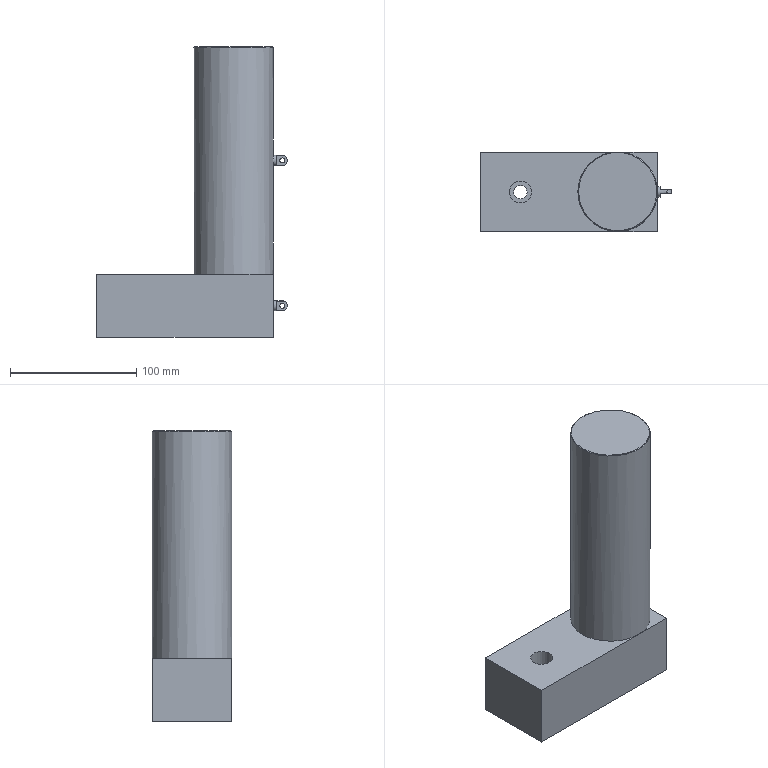Part | NX | features solid 2 | 1 solid | 37 faces | box 151 x 63 x 230 mm | volume 983981 mm3 | plane 23 | cylinder 13 | cone 1 | commonest cylinder face diameters 8 x4 4 x2 10.5 x2 17.5 x2 6 x1 10 x1
STEP:
#1=CARTESIAN_POINT('',(1540.,-559.,95.));
#2=VERTEX_POINT('',#1);
#3=CARTESIAN_POINT('',(1540.,-527.5,95.));
#4=VERTEX_POINT('',#3);
#5=CARTESIAN_POINT('',(1540.,-509.,95.));
#6=DIRECTION('',(0.,1.,0.));
#7=VECTOR('',#6,1000.);
#8=LINE('',#5,#7);
#9=EDGE_CURVE('',#2,#4,#8,.T.);
#10=ORIENTED_EDGE('',*,*,#9,.F.);
#11=CARTESIAN_POINT('',(1540.,-559.,45.));
#12=VERTEX_POINT('',#11);
#13=CARTESIAN_POINT('',(1540.,-559.,45.));
#14=DIRECTION('',(0.,0.,1.));
#15=VECTOR('',#14,1000.);
#16=LINE('',#13,#15);
#17=EDGE_CURVE('',#12,#2,#16,.T.);
#18=ORIENTED_EDGE('',*,*,#17,.F.);
#19=CARTESIAN_POINT('',(1540.,-496.,45.));
#20=VERTEX_POINT('',#19);
#21=CARTESIAN_POINT('',(1540.,-509.,45.));
#22=DIRECTION('',(0.,-1.,0.));
#23=VECTOR('',#22,1000.);
#24=LINE('',#21,#23);
#25=EDGE_CURVE('',#20,#12,#24,.T.);
#26=ORIENTED_EDGE('',*,*,#25,.F.);
#27=CARTESIAN_POINT('',(1540.,-496.,95.));
#28=VERTEX_POINT('',#27);
#29=CARTESIAN_POINT('',(1540.,-496.,203.412));
#30=DIRECTION('',(0.,0.,1.));
#31=VECTOR('',#30,1000.);
#32=LINE('',#29,#31);
#33=EDGE_CURVE('',#20,#28,#32,.T.);
#34=ORIENTED_EDGE('',*,*,#33,.T.);
#35=CARTESIAN_POINT('',(1540.,-509.,95.));
#36=DIRECTION('',(0.,1.,0.));
#37=VECTOR('',#36,1000.);
#38=LINE('',#35,#37);
#39=EDGE_CURVE('',#4,#28,#38,.T.);
#40=ORIENTED_EDGE('',*,*,#39,.F.);
#41=EDGE_LOOP('',(#10,#18,#26,#34,#40));
#42=FACE_BOUND('',#41,.T.);
#43=CARTESIAN_POINT('',(1540.,-523.5,70.));
#44=VERTEX_POINT('',#43);
#45=CARTESIAN_POINT('',(1540.,-527.5,70.));
#46=DIRECTION('',(1.,0.,0.));
#47=DIRECTION('',(0.,1.,0.));
#48=AXIS2_PLACEMENT_3D('',#45,#46,#47);
#49=CIRCLE('',#48,4.);
#50=EDGE_CURVE('',#44,#44,#49,.F.);
#51=ORIENTED_EDGE('',*,*,#50,.T.);
#52=EDGE_LOOP('',(#51));
#53=FACE_BOUND('',#52,.T.);
#54=CARTESIAN_POINT('',(1540.,-509.,45.));
#55=DIRECTION('',(1.,0.,0.));
#56=DIRECTION('',(0.,1.,0.));
#57=AXIS2_PLACEMENT_3D('',#54,#55,#56);
#58=PLANE('',#57);
#59=ADVANCED_FACE('',(#42,#53),#58,.T.);
#60=ORIENTED_EDGE('',*,*,#9,.T.);
#61=CARTESIAN_POINT('',(1508.5,-559.,95.));
#62=VERTEX_POINT('',#61);
#63=CARTESIAN_POINT('',(1508.5,-527.5,95.));
#64=DIRECTION('',(0.,0.,-1.));
#65=DIRECTION('',(1.,0.,0.));
#66=AXIS2_PLACEMENT_3D('',#63,#64,#65);
#67=CIRCLE('',#66,31.5);
#68=EDGE_CURVE('',#4,#62,#67,.T.);
#69=ORIENTED_EDGE('',*,*,#68,.T.);
#70=CARTESIAN_POINT('',(1263.352,-559.,95.));
#71=DIRECTION('',(1.,0.,0.));
#72=VECTOR('',#71,1000.);
#73=LINE('',#70,#72);
#74=EDGE_CURVE('',#62,#2,#73,.T.);
#75=ORIENTED_EDGE('',*,*,#74,.T.);
#76=EDGE_LOOP('',(#60,#69,#75));
#77=FACE_BOUND('',#76,.T.);
#78=CARTESIAN_POINT('',(1470.,-527.5,95.));
#79=DIRECTION('',(0.,0.,-1.));
#80=DIRECTION('',(1.,0.,0.));
#81=AXIS2_PLACEMENT_3D('',#78,#79,#80);
#82=PLANE('',#81);
#83=ADVANCED_FACE('',(#77),#82,.F.);
#84=CARTESIAN_POINT('',(1422.75,-527.5,95.));
#85=VERTEX_POINT('',#84);
#86=CARTESIAN_POINT('',(1431.5,-527.5,95.));
#87=DIRECTION('',(0.,0.,1.));
#88=DIRECTION('',(-1.,0.,0.));
#89=AXIS2_PLACEMENT_3D('',#86,#87,#88);
#90=CIRCLE('',#89,8.75);
#91=EDGE_CURVE('',#85,#85,#90,.F.);
#92=ORIENTED_EDGE('',*,*,#91,.T.);
#93=EDGE_LOOP('',(#92));
#94=FACE_BOUND('',#93,.T.);
#95=CARTESIAN_POINT('',(1400.,-559.,95.));
#96=VERTEX_POINT('',#95);
#97=CARTESIAN_POINT('',(1263.352,-559.,95.));
#98=DIRECTION('',(1.,0.,0.));
#99=VECTOR('',#98,1000.);
#100=LINE('',#97,#99);
#101=EDGE_CURVE('',#96,#62,#100,.T.);
#102=ORIENTED_EDGE('',*,*,#101,.T.);
#103=CARTESIAN_POINT('',(1508.5,-496.,95.));
#104=VERTEX_POINT('',#103);
#105=CARTESIAN_POINT('',(1508.5,-527.5,95.));
#106=DIRECTION('',(0.,0.,-1.));
#107=DIRECTION('',(1.,0.,0.));
#108=AXIS2_PLACEMENT_3D('',#105,#106,#107);
#109=CIRCLE('',#108,31.5);
#110=EDGE_CURVE('',#62,#104,#109,.T.);
#111=ORIENTED_EDGE('',*,*,#110,.T.);
#112=CARTESIAN_POINT('',(1400.,-496.,95.));
#113=VERTEX_POINT('',#112);
#114=CARTESIAN_POINT('',(1263.352,-496.,95.));
#115=DIRECTION('',(1.,0.,0.));
#116=VECTOR('',#115,1000.);
#117=LINE('',#114,#116);
#118=EDGE_CURVE('',#113,#104,#117,.T.);
#119=ORIENTED_EDGE('',*,*,#118,.F.);
#120=CARTESIAN_POINT('',(1400.,-509.,95.));
#121=DIRECTION('',(0.,1.,0.));
#122=VECTOR('',#121,1000.);
#123=LINE('',#120,#122);
#124=EDGE_CURVE('',#96,#113,#123,.T.);
#125=ORIENTED_EDGE('',*,*,#124,.F.);
#126=EDGE_LOOP('',(#102,#111,#119,#125));
#127=FACE_BOUND('',#126,.T.);
#128=CARTESIAN_POINT('',(1470.,-527.5,95.));
#129=DIRECTION('',(0.,0.,-1.));
#130=DIRECTION('',(1.,0.,0.));
#131=AXIS2_PLACEMENT_3D('',#128,#129,#130);
#132=PLANE('',#131);
#133=ADVANCED_FACE('',(#94,#127),#132,.F.);
#134=CARTESIAN_POINT('',(1400.,-496.,45.));
#135=VERTEX_POINT('',#134);
#136=CARTESIAN_POINT('',(1263.352,-496.,45.));
#137=DIRECTION('',(1.,0.,0.));
#138=VECTOR('',#137,1000.);
#139=LINE('',#136,#138);
#140=EDGE_CURVE('',#135,#20,#139,.T.);
#141=ORIENTED_EDGE('',*,*,#140,.F.);
#142=CARTESIAN_POINT('',(1400.,-496.,203.412));
#143=DIRECTION('',(0.,0.,1.));
#144=VECTOR('',#143,1000.);
#145=LINE('',#142,#144);
#146=EDGE_CURVE('',#135,#113,#145,.T.);
#147=ORIENTED_EDGE('',*,*,#146,.T.);
#148=ORIENTED_EDGE('',*,*,#118,.T.);
#149=CARTESIAN_POINT('',(1263.352,-496.,95.));
#150=DIRECTION('',(1.,0.,0.));
#151=VECTOR('',#150,1000.);
#152=LINE('',#149,#151);
#153=EDGE_CURVE('',#104,#28,#152,.T.);
#154=ORIENTED_EDGE('',*,*,#153,.T.);
#155=ORIENTED_EDGE('',*,*,#33,.F.);
#156=EDGE_LOOP('',(#141,#147,#148,#154,#155));
#157=FACE_BOUND('',#156,.T.);
#158=CARTESIAN_POINT('',(1263.352,-496.,203.412));
#159=DIRECTION('',(0.,-1.,0.));
#160=DIRECTION('',(1.,0.,0.));
#161=AXIS2_PLACEMENT_3D('',#158,#159,#160);
#162=PLANE('',#161);
#163=ADVANCED_FACE('',(#157),#162,.F.);
#164=ORIENTED_EDGE('',*,*,#101,.F.);
#165=CARTESIAN_POINT('',(1400.,-559.,45.));
#166=VERTEX_POINT('',#165);
#167=CARTESIAN_POINT('',(1400.,-559.,45.));
#168=DIRECTION('',(0.,0.,1.));
#169=VECTOR('',#168,1000.);
#170=LINE('',#167,#169);
#171=EDGE_CURVE('',#166,#96,#170,.T.);
#172=ORIENTED_EDGE('',*,*,#171,.F.);
#173=CARTESIAN_POINT('',(1263.352,-559.,45.));
#174=DIRECTION('',(1.,0.,0.));
#175=VECTOR('',#174,1000.);
#176=LINE('',#173,#175);
#177=EDGE_CURVE('',#166,#12,#176,.T.);
#178=ORIENTED_EDGE('',*,*,#177,.T.);
#179=ORIENTED_EDGE('',*,*,#17,.T.);
#180=ORIENTED_EDGE('',*,*,#74,.F.);
#181=EDGE_LOOP('',(#164,#172,#178,#179,#180));
#182=FACE_BOUND('',#181,.T.);
#183=CARTESIAN_POINT('',(1263.352,-559.,203.412));
#184=DIRECTION('',(0.,-1.,0.));
#185=DIRECTION('',(1.,0.,0.));
#186=AXIS2_PLACEMENT_3D('',#183,#184,#185);
#187=PLANE('',#186);
#188=ADVANCED_FACE('',(#182),#187,.T.);
#189=CARTESIAN_POINT('',(1513.75,-527.5,45.));
#190=VERTEX_POINT('',#189);
#191=CARTESIAN_POINT('',(1508.5,-527.5,45.));
#192=DIRECTION('',(0.,0.,-1.));
#193=DIRECTION('',(1.,0.,0.));
#194=AXIS2_PLACEMENT_3D('',#191,#192,#193);
#195=CIRCLE('',#194,5.25);
#196=EDGE_CURVE('',#190,#190,#195,.F.);
#197=ORIENTED_EDGE('',*,*,#196,.T.);
#198=EDGE_LOOP('',(#197));
#199=FACE_BOUND('',#198,.T.);
#200=ORIENTED_EDGE('',*,*,#25,.T.);
#201=ORIENTED_EDGE('',*,*,#177,.F.);
#202=CARTESIAN_POINT('',(1400.,-509.,45.));
#203=DIRECTION('',(0.,-1.,0.));
#204=VECTOR('',#203,1000.);
#205=LINE('',#202,#204);
#206=EDGE_CURVE('',#135,#166,#205,.T.);
#207=ORIENTED_EDGE('',*,*,#206,.F.);
#208=ORIENTED_EDGE('',*,*,#140,.T.);
#209=EDGE_LOOP('',(#200,#201,#207,#208));
#210=FACE_BOUND('',#209,.T.);
#211=CARTESIAN_POINT('',(1426.25,-527.5,45.));
#212=VERTEX_POINT('',#211);
#213=CARTESIAN_POINT('',(1431.5,-527.5,45.));
#214=DIRECTION('',(0.,0.,1.));
#215=DIRECTION('',(-1.,0.,0.));
#216=AXIS2_PLACEMENT_3D('',#213,#214,#215);
#217=CIRCLE('',#216,5.25);
#218=EDGE_CURVE('',#212,#212,#217,.F.);
#219=ORIENTED_EDGE('',*,*,#218,.F.);
#220=EDGE_LOOP('',(#219));
#221=FACE_BOUND('',#220,.T.);
#222=CARTESIAN_POINT('',(1263.352,-509.,45.));
#223=DIRECTION('',(0.,0.,-1.));
#224=DIRECTION('',(-1.,0.,0.));
#225=AXIS2_PLACEMENT_3D('',#222,#223,#224);
#226=PLANE('',#225);
#227=ADVANCED_FACE('',(#199,#210,#221),#226,.T.);
#228=ORIENTED_EDGE('',*,*,#153,.F.);
#229=CARTESIAN_POINT('',(1508.5,-527.5,95.));
#230=DIRECTION('',(0.,0.,-1.));
#231=DIRECTION('',(1.,0.,0.));
#232=AXIS2_PLACEMENT_3D('',#229,#230,#231);
#233=CIRCLE('',#232,31.5);
#234=EDGE_CURVE('',#104,#4,#233,.T.);
#235=ORIENTED_EDGE('',*,*,#234,.T.);
#236=ORIENTED_EDGE('',*,*,#39,.T.);
#237=EDGE_LOOP('',(#228,#235,#236));
#238=FACE_BOUND('',#237,.T.);
#239=CARTESIAN_POINT('',(1470.,-527.5,95.));
#240=DIRECTION('',(0.,0.,-1.));
#241=DIRECTION('',(1.,0.,0.));
#242=AXIS2_PLACEMENT_3D('',#239,#240,#241);
#243=PLANE('',#242);
#244=ADVANCED_FACE('',(#238),#243,.F.);
#245=CARTESIAN_POINT('',(1517.25,-527.5,65.));
#246=VERTEX_POINT('',#245);
#247=CARTESIAN_POINT('',(1508.5,-527.5,65.));
#248=DIRECTION('',(0.,0.,1.));
#249=DIRECTION('',(1.,0.,0.));
#250=AXIS2_PLACEMENT_3D('',#247,#248,#249);
#251=CIRCLE('',#250,8.75);
#252=EDGE_CURVE('',#246,#246,#251,.T.);
#253=ORIENTED_EDGE('',*,*,#252,.F.);
#254=EDGE_LOOP('',(#253));
#255=FACE_BOUND('',#254,.T.);
#256=CARTESIAN_POINT('',(1517.25,-527.5,95.));
#257=VERTEX_POINT('',#256);
#258=CARTESIAN_POINT('',(1508.5,-527.5,95.));
#259=DIRECTION('',(0.,0.,-1.));
#260=DIRECTION('',(1.,0.,0.));
#261=AXIS2_PLACEMENT_3D('',#258,#259,#260);
#262=CIRCLE('',#261,8.75);
#263=EDGE_CURVE('',#257,#257,#262,.F.);
#264=ORIENTED_EDGE('',*,*,#263,.T.);
#265=EDGE_LOOP('',(#264));
#266=FACE_BOUND('',#265,.T.);
#267=CARTESIAN_POINT('',(1508.5,-527.5,45.));
#268=DIRECTION('',(0.,0.,1.));
#269=DIRECTION('',(1.,0.,0.));
#270=AXIS2_PLACEMENT_3D('',#267,#268,#269);
#271=CYLINDRICAL_SURFACE('',#270,8.75);
#272=ADVANCED_FACE('',(#255,#266),#271,.F.);
#273=CARTESIAN_POINT('',(1513.75,-527.5,65.));
#274=VERTEX_POINT('',#273);
#275=CARTESIAN_POINT('',(1508.5,-527.5,65.));
#276=DIRECTION('',(0.,0.,-1.));
#277=DIRECTION('',(1.,0.,0.));
#278=AXIS2_PLACEMENT_3D('',#275,#276,#277);
#279=CIRCLE('',#278,5.25);
#280=EDGE_CURVE('',#274,#274,#279,.F.);
#281=ORIENTED_EDGE('',*,*,#280,.F.);
#282=EDGE_LOOP('',(#281));
#283=FACE_BOUND('',#282,.T.);
#284=ORIENTED_EDGE('',*,*,#252,.T.);
#285=EDGE_LOOP('',(#284));
#286=FACE_BOUND('',#285,.T.);
#287=CARTESIAN_POINT('',(1508.5,-527.5,65.));
#288=DIRECTION('',(0.,0.,-1.));
#289=DIRECTION('',(1.,0.,0.));
#290=AXIS2_PLACEMENT_3D('',#287,#288,#289);
#291=PLANE('',#290);
#292=ADVANCED_FACE('',(#283,#286),#291,.F.);
#293=ORIENTED_EDGE('',*,*,#196,.F.);
#294=EDGE_LOOP('',(#293));
#295=FACE_BOUND('',#294,.T.);
#296=ORIENTED_EDGE('',*,*,#280,.T.);
#297=EDGE_LOOP('',(#296));
#298=FACE_BOUND('',#297,.T.);
#299=CARTESIAN_POINT('',(1508.5,-527.5,65.));
#300=DIRECTION('',(0.,0.,-1.));
#301=DIRECTION('',(1.,0.,0.));
#302=AXIS2_PLACEMENT_3D('',#299,#300,#301);
#303=CYLINDRICAL_SURFACE('',#302,5.25);
#304=ADVANCED_FACE('',(#295,#298),#303,.F.);
#305=ORIENTED_EDGE('',*,*,#124,.T.);
#306=ORIENTED_EDGE('',*,*,#146,.F.);
#307=ORIENTED_EDGE('',*,*,#206,.T.);
#308=ORIENTED_EDGE('',*,*,#171,.T.);
#309=EDGE_LOOP('',(#305,#306,#307,#308));
#310=FACE_BOUND('',#309,.T.);
#311=CARTESIAN_POINT('',(1400.,-509.,45.));
#312=DIRECTION('',(-1.,0.,0.));
#313=DIRECTION('',(0.,1.,0.));
#314=AXIS2_PLACEMENT_3D('',#311,#312,#313);
#315=PLANE('',#314);
#316=ADVANCED_FACE('',(#310),#315,.T.);
#317=CARTESIAN_POINT('',(1422.75,-527.5,65.));
#318=VERTEX_POINT('',#317);
#319=CARTESIAN_POINT('',(1431.5,-527.5,65.));
#320=DIRECTION('',(0.,0.,-1.));
#321=DIRECTION('',(-1.,0.,0.));
#322=AXIS2_PLACEMENT_3D('',#319,#320,#321);
#323=CIRCLE('',#322,8.75);
#324=EDGE_CURVE('',#318,#318,#323,.T.);
#325=ORIENTED_EDGE('',*,*,#324,.T.);
#326=EDGE_LOOP('',(#325));
#327=FACE_BOUND('',#326,.T.);
#328=ORIENTED_EDGE('',*,*,#91,.F.);
#329=EDGE_LOOP('',(#328));
#330=FACE_BOUND('',#329,.T.);
#331=CARTESIAN_POINT('',(1431.5,-527.5,45.));
#332=DIRECTION('',(0.,0.,1.));
#333=DIRECTION('',(-1.,0.,0.));
#334=AXIS2_PLACEMENT_3D('',#331,#332,#333);
#335=CYLINDRICAL_SURFACE('',#334,8.75);
#336=ADVANCED_FACE('',(#327,#330),#335,.F.);
#337=CARTESIAN_POINT('',(1426.25,-527.5,65.));
#338=VERTEX_POINT('',#337);
#339=CARTESIAN_POINT('',(1431.5,-527.5,65.));
#340=DIRECTION('',(0.,0.,1.));
#341=DIRECTION('',(-1.,0.,0.));
#342=AXIS2_PLACEMENT_3D('',#339,#340,#341);
#343=CIRCLE('',#342,5.25);
#344=EDGE_CURVE('',#338,#338,#343,.F.);
#345=ORIENTED_EDGE('',*,*,#344,.T.);
#346=EDGE_LOOP('',(#345));
#347=FACE_BOUND('',#346,.T.);
#348=ORIENTED_EDGE('',*,*,#324,.F.);
#349=EDGE_LOOP('',(#348));
#350=FACE_BOUND('',#349,.T.);
#351=CARTESIAN_POINT('',(1431.5,-527.5,65.));
#352=DIRECTION('',(0.,0.,-1.));
#353=DIRECTION('',(-1.,0.,0.));
#354=AXIS2_PLACEMENT_3D('',#351,#352,#353);
#355=PLANE('',#354);
#356=ADVANCED_FACE('',(#347,#350),#355,.F.);
#357=ORIENTED_EDGE('',*,*,#218,.T.);
#358=EDGE_LOOP('',(#357));
#359=FACE_BOUND('',#358,.T.);
#360=ORIENTED_EDGE('',*,*,#344,.F.);
#361=EDGE_LOOP('',(#360));
#362=FACE_BOUND('',#361,.T.);
#363=CARTESIAN_POINT('',(1431.5,-527.5,65.));
#364=DIRECTION('',(0.,0.,-1.));
#365=DIRECTION('',(-1.,0.,0.));
#366=AXIS2_PLACEMENT_3D('',#363,#364,#365);
#367=CYLINDRICAL_SURFACE('',#366,5.25);
#368=ADVANCED_FACE('',(#359,#362),#367,.F.);
#369=CARTESIAN_POINT('',(1539.,-527.5,190.));
#370=VERTEX_POINT('',#369);
#371=CARTESIAN_POINT('',(1539.,-527.5,185.));
#372=DIRECTION('',(-1.,0.,0.));
#373=DIRECTION('',(0.,0.,1.));
#374=AXIS2_PLACEMENT_3D('',#371,#372,#373);
#375=CIRCLE('',#374,5.);
#376=EDGE_CURVE('',#370,#370,#375,.T.);
#377=ORIENTED_EDGE('',*,*,#376,.F.);
#378=EDGE_LOOP('',(#377));
#379=FACE_BOUND('',#378,.T.);
#380=CARTESIAN_POINT('',(1539.,-527.5,189.));
#381=VERTEX_POINT('',#380);
#382=CARTESIAN_POINT('',(1539.,-527.5,185.));
#383=DIRECTION('',(-1.,0.,0.));
#384=DIRECTION('',(0.,0.,1.));
#385=AXIS2_PLACEMENT_3D('',#382,#383,#384);
#386=CIRCLE('',#385,4.);
#387=EDGE_CURVE('',#381,#381,#386,.T.);
#388=ORIENTED_EDGE('',*,*,#387,.T.);
#389=EDGE_LOOP('',(#388));
#390=FACE_BOUND('',#389,.T.);
#391=CARTESIAN_POINT('',(1539.,-527.5,185.));
#392=DIRECTION('',(1.,0.,0.));
#393=DIRECTION('',(0.,0.,-1.));
#394=AXIS2_PLACEMENT_3D('',#391,#392,#393);
#395=PLANE('',#394);
#396=ADVANCED_FACE('',(#379,#390),#395,.T.);
#397=CARTESIAN_POINT('',(1540.,-527.5,274.5));
#398=VERTEX_POINT('',#397);
#399=CARTESIAN_POINT('',(1508.5,-527.5,274.5));
#400=DIRECTION('',(0.,0.,-1.));
#401=DIRECTION('',(1.,0.,0.));
#402=AXIS2_PLACEMENT_3D('',#399,#400,#401);
#403=CIRCLE('',#402,31.5);
#404=EDGE_CURVE('',#398,#398,#403,.F.);
#405=ORIENTED_EDGE('',*,*,#404,.F.);
#406=EDGE_LOOP('',(#405));
#407=FACE_BOUND('',#406,.T.);
#408=CARTESIAN_POINT('',(1540.,-527.5,180.));
#409=VERTEX_POINT('',#408);
#410=CARTESIAN_POINT('',(1539.801,-531.422,181.085));
#411=CARTESIAN_POINT('',(1540.099,-527.499,179.458));
#412=CARTESIAN_POINT('',(1539.801,-523.581,181.084));
#413=CARTESIAN_POINT('',(1539.5,-521.96,184.995));
#414=CARTESIAN_POINT('',(1539.801,-523.58,188.918));
#415=CARTESIAN_POINT('',(1540.099,-527.499,190.54));
#416=CARTESIAN_POINT('',(1539.802,-531.413,188.922));
#417=CARTESIAN_POINT('',(1539.5,-533.041,185.004));
#418=CARTESIAN_POINT('',(1539.801,-531.422,181.085));
#419=CARTESIAN_POINT('',(1540.099,-527.499,179.458));
#420=CARTESIAN_POINT('',(1539.801,-523.581,181.084));
#421=B_SPLINE_CURVE_WITH_KNOTS('',3,(#410,#411,#412,#413,#414,#415,#416,#417,#418,#419,#420),.UNSPECIFIED.,.T.,.F.,(1,1,1,1,1,1,1,1,1,1,1,1,1,1,1),(-0.01174,-0.007828,-0.003914,0.,0.003914,0.007828,0.01174,0.01566,0.01957,0.02348,0.0274,0.03131,0.03522,0.03914,0.04305),.UNSPECIFIED.);
#422=EDGE_CURVE('',#409,#409,#421,.T.);
#423=ORIENTED_EDGE('',*,*,#422,.F.);
#424=EDGE_LOOP('',(#423));
#425=FACE_BOUND('',#424,.T.);
#426=ORIENTED_EDGE('',*,*,#68,.F.);
#427=ORIENTED_EDGE('',*,*,#234,.F.);
#428=ORIENTED_EDGE('',*,*,#110,.F.);
#429=EDGE_LOOP('',(#426,#427,#428));
#430=FACE_BOUND('',#429,.T.);
#431=CARTESIAN_POINT('',(1508.5,-527.5,275.));
#432=DIRECTION('',(0.,0.,-1.));
#433=DIRECTION('',(-1.,0.,0.));
#434=AXIS2_PLACEMENT_3D('',#431,#432,#433);
#435=CYLINDRICAL_SURFACE('',#434,31.5);
#436=ADVANCED_FACE('',(#407,#425,#430),#435,.T.);
#437=CARTESIAN_POINT('',(1539.5,-527.5,275.));
#438=VERTEX_POINT('',#437);
#439=CARTESIAN_POINT('',(1508.5,-527.5,275.));
#440=DIRECTION('',(0.,0.,-1.));
#441=DIRECTION('',(1.,0.,0.));
#442=AXIS2_PLACEMENT_3D('',#439,#440,#441);
#443=CIRCLE('',#442,31.);
#444=EDGE_CURVE('',#438,#438,#443,.T.);
#445=ORIENTED_EDGE('',*,*,#444,.F.);
#446=EDGE_LOOP('',(#445));
#447=FACE_BOUND('',#446,.T.);
#448=CARTESIAN_POINT('',(1508.5,-527.5,275.));
#449=DIRECTION('',(0.,0.,1.));
#450=DIRECTION('',(1.,0.,0.));
#451=AXIS2_PLACEMENT_3D('',#448,#449,#450);
#452=PLANE('',#451);
#453=ADVANCED_FACE('',(#447),#452,.T.);
#454=ORIENTED_EDGE('',*,*,#376,.T.);
#455=EDGE_LOOP('',(#454));
#456=FACE_BOUND('',#455,.T.);
#457=ORIENTED_EDGE('',*,*,#422,.T.);
#458=EDGE_LOOP('',(#457));
#459=FACE_BOUND('',#458,.T.);
#460=CARTESIAN_POINT('',(1539.,-527.5,185.));
#461=DIRECTION('',(1.,0.,0.));
#462=DIRECTION('',(0.,0.,-1.));
#463=AXIS2_PLACEMENT_3D('',#460,#461,#462);
#464=CYLINDRICAL_SURFACE('',#463,5.);
#465=ADVANCED_FACE('',(#456,#459),#464,.F.);
#466=ORIENTED_EDGE('',*,*,#404,.T.);
#467=EDGE_LOOP('',(#466));
#468=FACE_BOUND('',#467,.T.);
#469=ORIENTED_EDGE('',*,*,#444,.T.);
#470=EDGE_LOOP('',(#469));
#471=FACE_BOUND('',#470,.T.);
#472=CARTESIAN_POINT('',(1508.5,-527.5,275.));
#473=DIRECTION('',(0.,0.,-1.));
#474=DIRECTION('',(-1.,0.,0.));
#475=AXIS2_PLACEMENT_3D('',#472,#473,#474);
#476=CONICAL_SURFACE('',#475,31.,0.7854);
#477=ADVANCED_FACE('',(#468,#471),#476,.T.);
#478=CARTESIAN_POINT('',(1548.5,-526.,181.292));
#479=VERTEX_POINT('',#478);
#480=CARTESIAN_POINT('',(1548.5,-526.,188.708));
#481=VERTEX_POINT('',#480);
#482=CARTESIAN_POINT('',(1547.,-526.,185.));
#483=DIRECTION('',(0.,-1.,0.));
#484=DIRECTION('',(1.,0.,0.));
#485=AXIS2_PLACEMENT_3D('',#482,#483,#484);
#486=CIRCLE('',#485,4.);
#487=EDGE_CURVE('',#479,#481,#486,.T.);
#488=ORIENTED_EDGE('',*,*,#487,.F.);
#489=CARTESIAN_POINT('',(1542.,-526.,181.292));
#490=VERTEX_POINT('',#489);
#491=CARTESIAN_POINT('',(1551.,-526.,181.292));
#492=DIRECTION('',(-1.,0.,0.));
#493=VECTOR('',#492,1000.);
#494=LINE('',#491,#493);
#495=EDGE_CURVE('',#490,#479,#494,.F.);
#496=ORIENTED_EDGE('',*,*,#495,.F.);
#497=CARTESIAN_POINT('',(1542.,-526.,188.708));
#498=VERTEX_POINT('',#497);
#499=CARTESIAN_POINT('',(1542.,-526.,189.));
#500=DIRECTION('',(0.,0.,-1.));
#501=VECTOR('',#500,1000.);
#502=LINE('',#499,#501);
#503=EDGE_CURVE('',#498,#490,#502,.T.);
#504=ORIENTED_EDGE('',*,*,#503,.F.);
#505=CARTESIAN_POINT('',(1551.,-526.,188.708));
#506=DIRECTION('',(-1.,0.,0.));
#507=VECTOR('',#506,1000.);
#508=LINE('',#505,#507);
#509=EDGE_CURVE('',#481,#498,#508,.T.);
#510=ORIENTED_EDGE('',*,*,#509,.F.);
#511=EDGE_LOOP('',(#488,#496,#504,#510));
#512=FACE_BOUND('',#511,.T.);
#513=CARTESIAN_POINT('',(1549.,-526.,185.));
#514=VERTEX_POINT('',#513);
#515=CARTESIAN_POINT('',(1547.,-526.,185.));
#516=DIRECTION('',(0.,-1.,0.));
#517=DIRECTION('',(1.,0.,0.));
#518=AXIS2_PLACEMENT_3D('',#515,#516,#517);
#519=CIRCLE('',#518,2.);
#520=EDGE_CURVE('',#514,#514,#519,.F.);
#521=ORIENTED_EDGE('',*,*,#520,.F.);
#522=EDGE_LOOP('',(#521));
#523=FACE_BOUND('',#522,.T.);
#524=CARTESIAN_POINT('',(1551.,-526.,189.));
#525=DIRECTION('',(0.,1.,0.));
#526=DIRECTION('',(1.,0.,0.));
#527=AXIS2_PLACEMENT_3D('',#524,#525,#526);
#528=PLANE('',#527);
#529=ADVANCED_FACE('',(#512,#523),#528,.T.);
#530=CARTESIAN_POINT('',(1548.5,-529.,188.708));
#531=VERTEX_POINT('',#530);
#532=CARTESIAN_POINT('',(1548.5,-529.,181.292));
#533=VERTEX_POINT('',#532);
#534=CARTESIAN_POINT('',(1547.,-529.,185.));
#535=DIRECTION('',(0.,1.,0.));
#536=DIRECTION('',(-1.,0.,0.));
#537=AXIS2_PLACEMENT_3D('',#534,#535,#536);
#538=CIRCLE('',#537,4.);
#539=EDGE_CURVE('',#531,#533,#538,.T.);
#540=ORIENTED_EDGE('',*,*,#539,.F.);
#541=CARTESIAN_POINT('',(1542.,-529.,188.708));
#542=VERTEX_POINT('',#541);
#543=CARTESIAN_POINT('',(1551.,-529.,188.708));
#544=DIRECTION('',(-1.,0.,0.));
#545=VECTOR('',#544,1000.);
#546=LINE('',#543,#545);
#547=EDGE_CURVE('',#542,#531,#546,.F.);
#548=ORIENTED_EDGE('',*,*,#547,.F.);
#549=CARTESIAN_POINT('',(1542.,-529.,181.292));
#550=VERTEX_POINT('',#549);
#551=CARTESIAN_POINT('',(1542.,-529.,189.));
#552=DIRECTION('',(0.,0.,-1.));
#553=VECTOR('',#552,1000.);
#554=LINE('',#551,#553);
#555=EDGE_CURVE('',#542,#550,#554,.T.);
#556=ORIENTED_EDGE('',*,*,#555,.T.);
#557=CARTESIAN_POINT('',(1551.,-529.,181.292));
#558=DIRECTION('',(-1.,0.,0.));
#559=VECTOR('',#558,1000.);
#560=LINE('',#557,#559);
#561=EDGE_CURVE('',#533,#550,#560,.T.);
#562=ORIENTED_EDGE('',*,*,#561,.F.);
#563=EDGE_LOOP('',(#540,#548,#556,#562));
#564=FACE_BOUND('',#563,.T.);
#565=CARTESIAN_POINT('',(1545.,-529.,185.));
#566=VERTEX_POINT('',#565);
#567=CARTESIAN_POINT('',(1547.,-529.,185.));
#568=DIRECTION('',(0.,1.,0.));
#569=DIRECTION('',(-1.,0.,0.));
#570=AXIS2_PLACEMENT_3D('',#567,#568,#569);
#571=CIRCLE('',#570,2.);
#572=EDGE_CURVE('',#566,#566,#571,.F.);
#573=ORIENTED_EDGE('',*,*,#572,.F.);
#574=EDGE_LOOP('',(#573));
#575=FACE_BOUND('',#574,.T.);
#576=CARTESIAN_POINT('',(1542.,-529.,189.));
#577=DIRECTION('',(0.,-1.,0.));
#578=DIRECTION('',(-1.,0.,0.));
#579=AXIS2_PLACEMENT_3D('',#576,#577,#578);
#580=PLANE('',#579);
#581=ADVANCED_FACE('',(#564,#575),#580,.T.);
#582=ORIENTED_EDGE('',*,*,#387,.F.);
#583=EDGE_LOOP('',(#582));
#584=FACE_BOUND('',#583,.T.);
#585=CARTESIAN_POINT('',(1542.,-527.5,185.));
#586=DIRECTION('',(-1.,0.,0.));
#587=DIRECTION('',(0.,0.,-1.));
#588=AXIS2_PLACEMENT_3D('',#585,#586,#587);
#589=CIRCLE('',#588,4.);
#590=EDGE_CURVE('',#498,#490,#589,.T.);
#591=ORIENTED_EDGE('',*,*,#590,.T.);
#592=ORIENTED_EDGE('',*,*,#495,.T.);
#593=CARTESIAN_POINT('',(1547.,-527.5,181.));
#594=VERTEX_POINT('',#593);
#595=CARTESIAN_POINT('',(1547.,-527.5,185.));
#596=DIRECTION('',(0.7071,-0.7071,0.));
#597=DIRECTION('',(-0.7071,-0.7071,0.));
#598=AXIS2_PLACEMENT_3D('',#595,#596,#597);
#599=ELLIPSE('',#598,5.657,4.);
#600=EDGE_CURVE('',#594,#479,#599,.T.);
#601=ORIENTED_EDGE('',*,*,#600,.F.);
#602=CARTESIAN_POINT('',(1547.,-527.5,185.));
#603=DIRECTION('',(0.7071,0.7071,0.));
#604=DIRECTION('',(-0.7071,0.7071,0.));
#605=AXIS2_PLACEMENT_3D('',#602,#603,#604);
#606=ELLIPSE('',#605,5.657,4.);
#607=EDGE_CURVE('',#533,#594,#606,.T.);
#608=ORIENTED_EDGE('',*,*,#607,.F.);
#609=ORIENTED_EDGE('',*,*,#561,.T.);
#610=CARTESIAN_POINT('',(1542.,-527.5,185.));
#611=DIRECTION('',(-1.,0.,0.));
#612=DIRECTION('',(0.,0.,-1.));
#613=AXIS2_PLACEMENT_3D('',#610,#611,#612);
#614=CIRCLE('',#613,4.);
#615=EDGE_CURVE('',#550,#542,#614,.T.);
#616=ORIENTED_EDGE('',*,*,#615,.T.);
#617=ORIENTED_EDGE('',*,*,#547,.T.);
#618=CARTESIAN_POINT('',(1547.,-527.5,189.));
#619=VERTEX_POINT('',#618);
#620=CARTESIAN_POINT('',(1547.,-527.5,185.));
#621=DIRECTION('',(0.7071,0.7071,0.));
#622=DIRECTION('',(-0.7071,0.7071,0.));
#623=AXIS2_PLACEMENT_3D('',#620,#621,#622);
#624=ELLIPSE('',#623,5.657,4.);
#625=EDGE_CURVE('',#619,#531,#624,.T.);
#626=ORIENTED_EDGE('',*,*,#625,.F.);
#627=CARTESIAN_POINT('',(1547.,-527.5,185.));
#628=DIRECTION('',(0.7071,-0.7071,0.));
#629=DIRECTION('',(-0.7071,-0.7071,0.));
#630=AXIS2_PLACEMENT_3D('',#627,#628,#629);
#631=ELLIPSE('',#630,5.657,4.);
#632=EDGE_CURVE('',#481,#619,#631,.T.);
#633=ORIENTED_EDGE('',*,*,#632,.F.);
#634=ORIENTED_EDGE('',*,*,#509,.T.);
#635=EDGE_LOOP('',(#591,#592,#601,#608,#609,#616,#617,#626,#633,#634));
#636=FACE_BOUND('',#635,.T.);
#637=CARTESIAN_POINT('',(1551.,-527.5,185.));
#638=DIRECTION('',(-1.,0.,0.));
#639=DIRECTION('',(0.,0.,1.));
#640=AXIS2_PLACEMENT_3D('',#637,#638,#639);
#641=CYLINDRICAL_SURFACE('',#640,4.);
#642=ADVANCED_FACE('',(#584,#636),#641,.T.);
#643=ORIENTED_EDGE('',*,*,#539,.T.);
#644=ORIENTED_EDGE('',*,*,#607,.T.);
#645=ORIENTED_EDGE('',*,*,#600,.T.);
#646=ORIENTED_EDGE('',*,*,#487,.T.);
#647=ORIENTED_EDGE('',*,*,#632,.T.);
#648=ORIENTED_EDGE('',*,*,#625,.T.);
#649=EDGE_LOOP('',(#643,#644,#645,#646,#647,#648));
#650=FACE_BOUND('',#649,.T.);
#651=CARTESIAN_POINT('',(1547.,-519.5,185.));
#652=DIRECTION('',(0.,-1.,0.));
#653=DIRECTION('',(0.,0.,1.));
#654=AXIS2_PLACEMENT_3D('',#651,#652,#653);
#655=CYLINDRICAL_SURFACE('',#654,4.);
#656=ADVANCED_FACE('',(#650),#655,.T.);
#657=ORIENTED_EDGE('',*,*,#503,.T.);
#658=ORIENTED_EDGE('',*,*,#590,.F.);
#659=EDGE_LOOP('',(#657,#658));
#660=FACE_BOUND('',#659,.T.);
#661=CARTESIAN_POINT('',(1542.,-526.,189.));
#662=DIRECTION('',(1.,0.,0.));
#663=DIRECTION('',(0.,0.,-1.));
#664=AXIS2_PLACEMENT_3D('',#661,#662,#663);
#665=PLANE('',#664);
#666=ADVANCED_FACE('',(#660),#665,.T.);
#667=ORIENTED_EDGE('',*,*,#555,.F.);
#668=ORIENTED_EDGE('',*,*,#615,.F.);
#669=EDGE_LOOP('',(#667,#668));
#670=FACE_BOUND('',#669,.T.);
#671=CARTESIAN_POINT('',(1542.,-531.5,189.));
#672=DIRECTION('',(1.,0.,0.));
#673=DIRECTION('',(0.,0.,-1.));
#674=AXIS2_PLACEMENT_3D('',#671,#672,#673);
#675=PLANE('',#674);
#676=ADVANCED_FACE('',(#670),#675,.T.);
#677=ORIENTED_EDGE('',*,*,#520,.T.);
#678=EDGE_LOOP('',(#677));
#679=FACE_BOUND('',#678,.T.);
#680=ORIENTED_EDGE('',*,*,#572,.T.);
#681=EDGE_LOOP('',(#680));
#682=FACE_BOUND('',#681,.T.);
#683=CARTESIAN_POINT('',(1547.,-525.5,185.));
#684=DIRECTION('',(0.,-1.,0.));
#685=DIRECTION('',(0.,0.,1.));
#686=AXIS2_PLACEMENT_3D('',#683,#684,#685);
#687=CYLINDRICAL_SURFACE('',#686,2.);
#688=ADVANCED_FACE('',(#679,#682),#687,.F.);
#689=ORIENTED_EDGE('',*,*,#263,.F.);
#690=EDGE_LOOP('',(#689));
#691=FACE_BOUND('',#690,.T.);
#692=CARTESIAN_POINT('',(1508.5,-527.5,95.));
#693=DIRECTION('',(0.,0.,1.));
#694=DIRECTION('',(1.,0.,0.));
#695=AXIS2_PLACEMENT_3D('',#692,#693,#694);
#696=PLANE('',#695);
#697=ADVANCED_FACE('',(#691),#696,.F.);
#698=CARTESIAN_POINT('',(1545.,-529.,70.));
#699=VERTEX_POINT('',#698);
#700=CARTESIAN_POINT('',(1547.,-529.,70.));
#701=DIRECTION('',(0.,1.,0.));
#702=DIRECTION('',(-1.,0.,0.));
#703=AXIS2_PLACEMENT_3D('',#700,#701,#702);
#704=CIRCLE('',#703,2.);
#705=EDGE_CURVE('',#699,#699,#704,.T.);
#706=ORIENTED_EDGE('',*,*,#705,.F.);
#707=EDGE_LOOP('',(#706));
#708=FACE_BOUND('',#707,.T.);
#709=CARTESIAN_POINT('',(1549.,-526.,70.));
#710=VERTEX_POINT('',#709);
#711=CARTESIAN_POINT('',(1547.,-526.,70.));
#712=DIRECTION('',(0.,-1.,0.));
#713=DIRECTION('',(1.,0.,0.));
#714=AXIS2_PLACEMENT_3D('',#711,#712,#713);
#715=CIRCLE('',#714,2.);
#716=EDGE_CURVE('',#710,#710,#715,.T.);
#717=ORIENTED_EDGE('',*,*,#716,.F.);
#718=EDGE_LOOP('',(#717));
#719=FACE_BOUND('',#718,.T.);
#720=CARTESIAN_POINT('',(1547.,-519.5,70.));
#721=DIRECTION('',(0.,-1.,0.));
#722=DIRECTION('',(0.,0.,1.));
#723=AXIS2_PLACEMENT_3D('',#720,#721,#722);
#724=CYLINDRICAL_SURFACE('',#723,2.);
#725=ADVANCED_FACE('',(#708,#719),#724,.F.);
#726=CARTESIAN_POINT('',(1542.,-529.,73.708));
#727=VERTEX_POINT('',#726);
#728=CARTESIAN_POINT('',(1542.,-529.,66.292));
#729=VERTEX_POINT('',#728);
#730=CARTESIAN_POINT('',(1542.,-529.,75.));
#731=DIRECTION('',(0.,0.,-1.));
#732=VECTOR('',#731,1000.);
#733=LINE('',#730,#732);
#734=EDGE_CURVE('',#727,#729,#733,.T.);
#735=ORIENTED_EDGE('',*,*,#734,.F.);
#736=CARTESIAN_POINT('',(1542.,-527.5,70.));
#737=DIRECTION('',(-1.,0.,0.));
#738=DIRECTION('',(0.,0.,-1.));
#739=AXIS2_PLACEMENT_3D('',#736,#737,#738);
#740=CIRCLE('',#739,4.);
#741=EDGE_CURVE('',#729,#727,#740,.T.);
#742=ORIENTED_EDGE('',*,*,#741,.F.);
#743=EDGE_LOOP('',(#735,#742));
#744=FACE_BOUND('',#743,.T.);
#745=CARTESIAN_POINT('',(1542.,-531.5,75.));
#746=DIRECTION('',(1.,0.,0.));
#747=DIRECTION('',(0.,0.,-1.));
#748=AXIS2_PLACEMENT_3D('',#745,#746,#747);
#749=PLANE('',#748);
#750=ADVANCED_FACE('',(#744),#749,.T.);
#751=ORIENTED_EDGE('',*,*,#705,.T.);
#752=EDGE_LOOP('',(#751));
#753=FACE_BOUND('',#752,.T.);
#754=CARTESIAN_POINT('',(1548.5,-529.,73.708));
#755=VERTEX_POINT('',#754);
#756=CARTESIAN_POINT('',(1548.5,-529.,66.292));
#757=VERTEX_POINT('',#756);
#758=CARTESIAN_POINT('',(1547.,-529.,70.));
#759=DIRECTION('',(0.,1.,0.));
#760=DIRECTION('',(-1.,0.,0.));
#761=AXIS2_PLACEMENT_3D('',#758,#759,#760);
#762=CIRCLE('',#761,4.);
#763=EDGE_CURVE('',#755,#757,#762,.T.);
#764=ORIENTED_EDGE('',*,*,#763,.F.);
#765=CARTESIAN_POINT('',(1551.,-529.,73.708));
#766=DIRECTION('',(-1.,0.,0.));
#767=VECTOR('',#766,1000.);
#768=LINE('',#765,#767);
#769=EDGE_CURVE('',#727,#755,#768,.F.);
#770=ORIENTED_EDGE('',*,*,#769,.F.);
#771=ORIENTED_EDGE('',*,*,#734,.T.);
#772=CARTESIAN_POINT('',(1551.,-529.,66.292));
#773=DIRECTION('',(-1.,0.,0.));
#774=VECTOR('',#773,1000.);
#775=LINE('',#772,#774);
#776=EDGE_CURVE('',#757,#729,#775,.T.);
#777=ORIENTED_EDGE('',*,*,#776,.F.);
#778=EDGE_LOOP('',(#764,#770,#771,#777));
#779=FACE_BOUND('',#778,.T.);
#780=CARTESIAN_POINT('',(1542.,-529.,75.));
#781=DIRECTION('',(0.,-1.,0.));
#782=DIRECTION('',(-1.,0.,0.));
#783=AXIS2_PLACEMENT_3D('',#780,#781,#782);
#784=PLANE('',#783);
#785=ADVANCED_FACE('',(#753,#779),#784,.T.);
#786=ORIENTED_EDGE('',*,*,#763,.T.);
#787=CARTESIAN_POINT('',(1547.,-527.5,66.));
#788=VERTEX_POINT('',#787);
#789=CARTESIAN_POINT('',(1547.,-527.5,70.));
#790=DIRECTION('',(0.7071,0.7071,0.));
#791=DIRECTION('',(-0.7071,0.7071,0.));
#792=AXIS2_PLACEMENT_3D('',#789,#790,#791);
#793=ELLIPSE('',#792,5.657,4.);
#794=EDGE_CURVE('',#757,#788,#793,.T.);
#795=ORIENTED_EDGE('',*,*,#794,.T.);
#796=CARTESIAN_POINT('',(1548.5,-526.,66.292));
#797=VERTEX_POINT('',#796);
#798=CARTESIAN_POINT('',(1547.,-527.5,70.));
#799=DIRECTION('',(0.7071,-0.7071,0.));
#800=DIRECTION('',(-0.7071,-0.7071,0.));
#801=AXIS2_PLACEMENT_3D('',#798,#799,#800);
#802=ELLIPSE('',#801,5.657,4.);
#803=EDGE_CURVE('',#788,#797,#802,.T.);
#804=ORIENTED_EDGE('',*,*,#803,.T.);
#805=CARTESIAN_POINT('',(1548.5,-526.,73.708));
#806=VERTEX_POINT('',#805);
#807=CARTESIAN_POINT('',(1547.,-526.,70.));
#808=DIRECTION('',(0.,-1.,0.));
#809=DIRECTION('',(1.,0.,0.));
#810=AXIS2_PLACEMENT_3D('',#807,#808,#809);
#811=CIRCLE('',#810,4.);
#812=EDGE_CURVE('',#797,#806,#811,.T.);
#813=ORIENTED_EDGE('',*,*,#812,.T.);
#814=CARTESIAN_POINT('',(1547.,-527.5,74.));
#815=VERTEX_POINT('',#814);
#816=CARTESIAN_POINT('',(1547.,-527.5,70.));
#817=DIRECTION('',(0.7071,-0.7071,0.));
#818=DIRECTION('',(-0.7071,-0.7071,0.));
#819=AXIS2_PLACEMENT_3D('',#816,#817,#818);
#820=ELLIPSE('',#819,5.657,4.);
#821=EDGE_CURVE('',#806,#815,#820,.T.);
#822=ORIENTED_EDGE('',*,*,#821,.T.);
#823=CARTESIAN_POINT('',(1547.,-527.5,70.));
#824=DIRECTION('',(0.7071,0.7071,0.));
#825=DIRECTION('',(-0.7071,0.7071,0.));
#826=AXIS2_PLACEMENT_3D('',#823,#824,#825);
#827=ELLIPSE('',#826,5.657,4.);
#828=EDGE_CURVE('',#815,#755,#827,.T.);
#829=ORIENTED_EDGE('',*,*,#828,.T.);
#830=EDGE_LOOP('',(#786,#795,#804,#813,#822,#829));
#831=FACE_BOUND('',#830,.T.);
#832=CARTESIAN_POINT('',(1547.,-519.5,70.));
#833=DIRECTION('',(0.,-1.,0.));
#834=DIRECTION('',(0.,0.,1.));
#835=AXIS2_PLACEMENT_3D('',#832,#833,#834);
#836=CYLINDRICAL_SURFACE('',#835,4.);
#837=ADVANCED_FACE('',(#831),#836,.T.);
#838=ORIENTED_EDGE('',*,*,#716,.T.);
#839=EDGE_LOOP('',(#838));
#840=FACE_BOUND('',#839,.T.);
#841=ORIENTED_EDGE('',*,*,#812,.F.);
#842=CARTESIAN_POINT('',(1542.,-526.,66.292));
#843=VERTEX_POINT('',#842);
#844=CARTESIAN_POINT('',(1551.,-526.,66.292));
#845=DIRECTION('',(-1.,0.,0.));
#846=VECTOR('',#845,1000.);
#847=LINE('',#844,#846);
#848=EDGE_CURVE('',#843,#797,#847,.F.);
#849=ORIENTED_EDGE('',*,*,#848,.F.);
#850=CARTESIAN_POINT('',(1542.,-526.,73.708));
#851=VERTEX_POINT('',#850);
#852=CARTESIAN_POINT('',(1542.,-526.,75.));
#853=DIRECTION('',(0.,0.,-1.));
#854=VECTOR('',#853,1000.);
#855=LINE('',#852,#854);
#856=EDGE_CURVE('',#851,#843,#855,.T.);
#857=ORIENTED_EDGE('',*,*,#856,.F.);
#858=CARTESIAN_POINT('',(1551.,-526.,73.708));
#859=DIRECTION('',(-1.,0.,0.));
#860=VECTOR('',#859,1000.);
#861=LINE('',#858,#860);
#862=EDGE_CURVE('',#806,#851,#861,.T.);
#863=ORIENTED_EDGE('',*,*,#862,.F.);
#864=EDGE_LOOP('',(#841,#849,#857,#863));
#865=FACE_BOUND('',#864,.T.);
#866=CARTESIAN_POINT('',(1551.,-526.,75.));
#867=DIRECTION('',(0.,1.,0.));
#868=DIRECTION('',(1.,0.,0.));
#869=AXIS2_PLACEMENT_3D('',#866,#867,#868);
#870=PLANE('',#869);
#871=ADVANCED_FACE('',(#840,#865),#870,.T.);
#872=ORIENTED_EDGE('',*,*,#856,.T.);
#873=CARTESIAN_POINT('',(1542.,-527.5,70.));
#874=DIRECTION('',(-1.,0.,0.));
#875=DIRECTION('',(0.,0.,-1.));
#876=AXIS2_PLACEMENT_3D('',#873,#874,#875);
#877=CIRCLE('',#876,4.);
#878=EDGE_CURVE('',#851,#843,#877,.T.);
#879=ORIENTED_EDGE('',*,*,#878,.F.);
#880=EDGE_LOOP('',(#872,#879));
#881=FACE_BOUND('',#880,.T.);
#882=CARTESIAN_POINT('',(1542.,-526.,75.));
#883=DIRECTION('',(1.,0.,0.));
#884=DIRECTION('',(0.,0.,-1.));
#885=AXIS2_PLACEMENT_3D('',#882,#883,#884);
#886=PLANE('',#885);
#887=ADVANCED_FACE('',(#881),#886,.T.);
#888=ORIENTED_EDGE('',*,*,#50,.F.);
#889=EDGE_LOOP('',(#888));
#890=FACE_BOUND('',#889,.T.);
#891=ORIENTED_EDGE('',*,*,#878,.T.);
#892=ORIENTED_EDGE('',*,*,#848,.T.);
#893=ORIENTED_EDGE('',*,*,#803,.F.);
#894=ORIENTED_EDGE('',*,*,#794,.F.);
#895=ORIENTED_EDGE('',*,*,#776,.T.);
#896=ORIENTED_EDGE('',*,*,#741,.T.);
#897=ORIENTED_EDGE('',*,*,#769,.T.);
#898=ORIENTED_EDGE('',*,*,#828,.F.);
#899=ORIENTED_EDGE('',*,*,#821,.F.);
#900=ORIENTED_EDGE('',*,*,#862,.T.);
#901=EDGE_LOOP('',(#891,#892,#893,#894,#895,#896,#897,#898,#899,#900));
#902=FACE_BOUND('',#901,.T.);
#903=CARTESIAN_POINT('',(1551.,-527.5,70.));
#904=DIRECTION('',(-1.,0.,0.));
#905=DIRECTION('',(0.,0.,1.));
#906=AXIS2_PLACEMENT_3D('',#903,#904,#905);
#907=CYLINDRICAL_SURFACE('',#906,4.);
#908=ADVANCED_FACE('',(#890,#902),#907,.T.);
#909=CLOSED_SHELL('',(#59,#83,#133,#163,#188,#227,#244,#272,#292,#304,#316,#336,#356,#368,#396,#436,#453,#465,#477,#529,#581,#642,#656,#666,#676,#688,#697,#725,#750,#785,#837,#871,#887,#908));
#910=CARTESIAN_POINT('',(1532.,-527.5,182.));
#911=VERTEX_POINT('',#910);
#912=CARTESIAN_POINT('',(1532.,-527.5,185.));
#913=DIRECTION('',(-1.,0.,0.));
#914=DIRECTION('',(0.,0.,-1.));
#915=AXIS2_PLACEMENT_3D('',#912,#913,#914);
#916=CIRCLE('',#915,3.);
#917=EDGE_CURVE('',#911,#911,#916,.F.);
#918=ORIENTED_EDGE('',*,*,#917,.F.);
#919=EDGE_LOOP('',(#918));
#920=FACE_BOUND('',#919,.T.);
#921=CARTESIAN_POINT('',(1532.,-527.5,185.));
#922=DIRECTION('',(1.,0.,0.));
#923=DIRECTION('',(0.,0.,-1.));
#924=AXIS2_PLACEMENT_3D('',#921,#922,#923);
#925=PLANE('',#924);
#926=ADVANCED_FACE('',(#920),#925,.F.);
#927=CARTESIAN_POINT('',(1507.5,-527.5,188.));
#928=VERTEX_POINT('',#927);
#929=CARTESIAN_POINT('',(1507.5,-527.5,185.));
#930=DIRECTION('',(1.,0.,0.));
#931=DIRECTION('',(0.,0.,1.));
#932=AXIS2_PLACEMENT_3D('',#929,#930,#931);
#933=CIRCLE('',#932,3.);
#934=EDGE_CURVE('',#928,#928,#933,.T.);
#935=ORIENTED_EDGE('',*,*,#934,.T.);
#936=EDGE_LOOP('',(#935));
#937=FACE_BOUND('',#936,.T.);
#938=CARTESIAN_POINT('',(1507.5,-527.5,185.));
#939=DIRECTION('',(-1.,0.,0.));
#940=DIRECTION('',(0.,0.,1.));
#941=AXIS2_PLACEMENT_3D('',#938,#939,#940);
#942=PLANE('',#941);
#943=ADVANCED_FACE('',(#937),#942,.F.);
#944=ORIENTED_EDGE('',*,*,#934,.F.);
#945=EDGE_LOOP('',(#944));
#946=FACE_BOUND('',#945,.T.);
#947=ORIENTED_EDGE('',*,*,#917,.T.);
#948=EDGE_LOOP('',(#947));
#949=FACE_BOUND('',#948,.T.);
#950=CARTESIAN_POINT('',(1539.,-527.5,185.));
#951=DIRECTION('',(-1.,0.,0.));
#952=DIRECTION('',(0.,0.,1.));
#953=AXIS2_PLACEMENT_3D('',#950,#951,#952);
#954=CYLINDRICAL_SURFACE('',#953,3.);
#955=ADVANCED_FACE('',(#946,#949),#954,.F.);
#956=CLOSED_SHELL('',(#926,#943,#955));
#957=ORIENTED_CLOSED_SHELL('',*,#956,.F.);
#958=BREP_WITH_VOIDS('',#909,(#957));
#959=(LENGTH_UNIT()NAMED_UNIT(*)SI_UNIT(.MILLI.,.METRE.));
#960=UNCERTAINTY_MEASURE_WITH_UNIT(LENGTH_MEASURE(0.0508),#959,'','');
#961=(NAMED_UNIT(*)PLANE_ANGLE_UNIT()SI_UNIT($,.RADIAN.));
#962=(NAMED_UNIT(*)SI_UNIT($,.STERADIAN.)SOLID_ANGLE_UNIT());
#963=(GEOMETRIC_REPRESENTATION_CONTEXT(3)GLOBAL_UNCERTAINTY_ASSIGNED_CONTEXT((#960))GLOBAL_UNIT_ASSIGNED_CONTEXT((#959,#961,#962))REPRESENTATION_CONTEXT('',''));
#964=ADVANCED_BREP_SHAPE_REPRESENTATION('',(#958),#963);